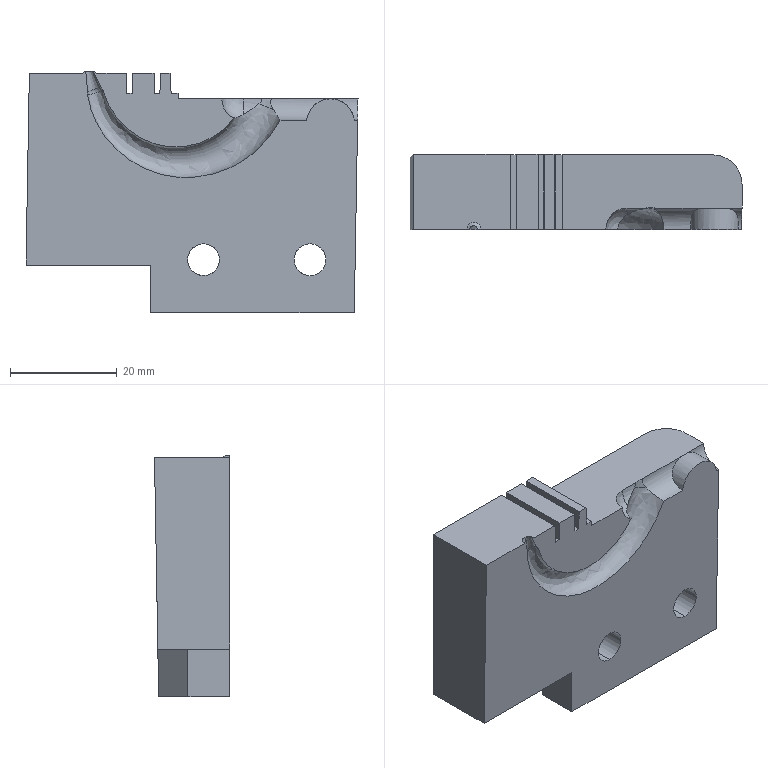Part | Creo | 1 solid | 156 faces | box 62.341 x 14.088 x 45.424 mm | volume 30917 mm3 | other 79 | plane 61 | cylinder 10 | sphere 3 | spline 2 | cone 1 | commonest cylinder face diameters 6 x4 8 x3 9 x1 11 x1 45.582 x1